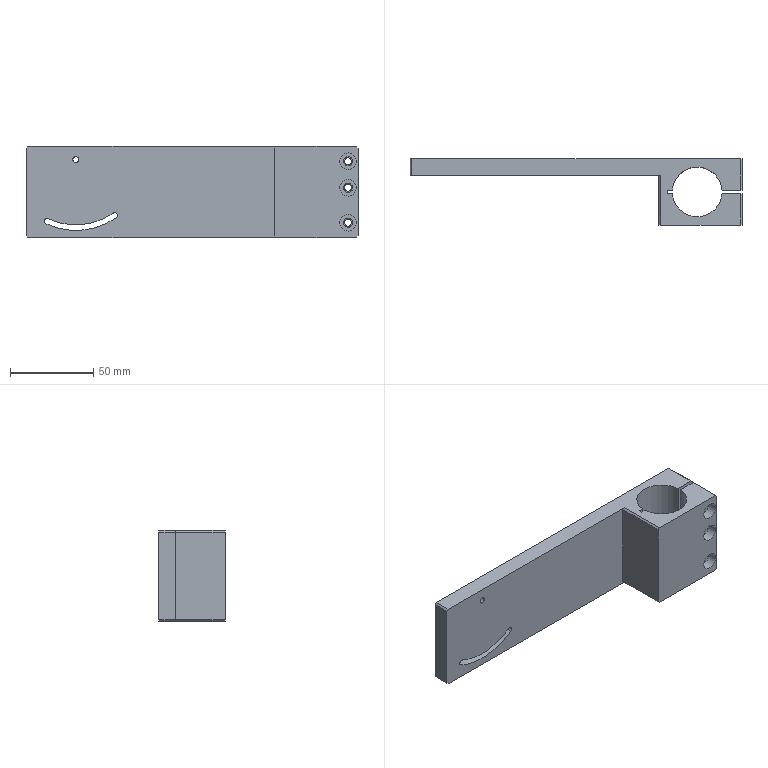Part | 1 solid | 41 faces | box 200 x 40 x 55 mm | volume 147214 mm3 | plane 25 | cylinder 16 | commonest cylinder face diameters 4.2 x3 5.5 x3 10 x3 3.3 x2 30 x2 3.5 x1
STEP:
#1=CARTESIAN_POINT('',(51.,10.,0.));
#2=VERTEX_POINT('',#1);
#3=CARTESIAN_POINT('',(50.,10.,1.));
#4=VERTEX_POINT('',#3);
#5=CARTESIAN_POINT('',(53.5,10.,-2.5));
#6=DIRECTION('',(-0.7071,0.,0.7071));
#7=VECTOR('',#6,1000.);
#8=LINE('',#5,#7);
#9=EDGE_CURVE('',#2,#4,#8,.T.);
#10=ORIENTED_EDGE('',*,*,#9,.F.);
#11=CARTESIAN_POINT('',(51.,-20.,0.));
#12=VERTEX_POINT('',#11);
#13=CARTESIAN_POINT('',(51.,10.,0.));
#14=DIRECTION('',(0.,1.,0.));
#15=VECTOR('',#14,1000.);
#16=LINE('',#13,#15);
#17=EDGE_CURVE('',#12,#2,#16,.T.);
#18=ORIENTED_EDGE('',*,*,#17,.F.);
#19=CARTESIAN_POINT('',(50.,-20.,1.));
#20=VERTEX_POINT('',#19);
#21=CARTESIAN_POINT('',(50.,-20.,1.));
#22=DIRECTION('',(0.7071,0.,-0.7071));
#23=VECTOR('',#22,1000.);
#24=LINE('',#21,#23);
#25=EDGE_CURVE('',#20,#12,#24,.T.);
#26=ORIENTED_EDGE('',*,*,#25,.F.);
#27=CARTESIAN_POINT('',(50.,-20.,1.));
#28=DIRECTION('',(0.,-1.,0.));
#29=VECTOR('',#28,1000.);
#30=LINE('',#27,#29);
#31=EDGE_CURVE('',#4,#20,#30,.T.);
#32=ORIENTED_EDGE('',*,*,#31,.F.);
#33=EDGE_LOOP('',(#10,#18,#26,#32));
#34=FACE_BOUND('',#33,.T.);
#35=CARTESIAN_POINT('',(50.,-20.,1.));
#36=DIRECTION('',(-0.7071,0.,-0.7071));
#37=DIRECTION('',(0.,1.,0.));
#38=AXIS2_PLACEMENT_3D('',#35,#36,#37);
#39=PLANE('',#38);
#40=ADVANCED_FACE('',(#34),#39,.T.);
#41=CARTESIAN_POINT('',(51.,-20.,55.));
#42=VERTEX_POINT('',#41);
#43=CARTESIAN_POINT('',(50.,-20.,54.));
#44=VERTEX_POINT('',#43);
#45=CARTESIAN_POINT('',(50.,-20.,54.));
#46=DIRECTION('',(-0.7071,0.,-0.7071));
#47=VECTOR('',#46,1000.);
#48=LINE('',#45,#47);
#49=EDGE_CURVE('',#42,#44,#48,.T.);
#50=ORIENTED_EDGE('',*,*,#49,.F.);
#51=CARTESIAN_POINT('',(51.,10.,55.));
#52=VERTEX_POINT('',#51);
#53=CARTESIAN_POINT('',(51.,0.,55.));
#54=DIRECTION('',(0.,-1.,0.));
#55=VECTOR('',#54,1000.);
#56=LINE('',#53,#55);
#57=EDGE_CURVE('',#52,#42,#56,.T.);
#58=ORIENTED_EDGE('',*,*,#57,.F.);
#59=CARTESIAN_POINT('',(50.,10.,54.));
#60=VERTEX_POINT('',#59);
#61=CARTESIAN_POINT('',(20.,10.,24.));
#62=DIRECTION('',(0.7071,0.,0.7071));
#63=VECTOR('',#62,1000.);
#64=LINE('',#61,#63);
#65=EDGE_CURVE('',#60,#52,#64,.T.);
#66=ORIENTED_EDGE('',*,*,#65,.F.);
#67=CARTESIAN_POINT('',(50.,-20.,54.));
#68=DIRECTION('',(0.,1.,0.));
#69=VECTOR('',#68,1000.);
#70=LINE('',#67,#69);
#71=EDGE_CURVE('',#44,#60,#70,.T.);
#72=ORIENTED_EDGE('',*,*,#71,.F.);
#73=EDGE_LOOP('',(#50,#58,#66,#72));
#74=FACE_BOUND('',#73,.T.);
#75=CARTESIAN_POINT('',(50.,-20.,54.));
#76=DIRECTION('',(0.7071,0.,-0.7071));
#77=DIRECTION('',(0.,1.,0.));
#78=AXIS2_PLACEMENT_3D('',#75,#76,#77);
#79=PLANE('',#78);
#80=ADVANCED_FACE('',(#74),#79,.F.);
#81=CARTESIAN_POINT('',(-47.441,20.,14.783));
#82=VERTEX_POINT('',#81);
#83=CARTESIAN_POINT('',(-47.441,10.,14.783));
#84=VERTEX_POINT('',#83);
#85=CARTESIAN_POINT('',(-47.441,71.,14.783));
#86=DIRECTION('',(0.,-1.,0.));
#87=VECTOR('',#86,1000.);
#88=LINE('',#85,#87);
#89=EDGE_CURVE('',#82,#84,#88,.T.);
#90=ORIENTED_EDGE('',*,*,#89,.T.);
#91=CARTESIAN_POINT('',(-86.622,10.,11.355));
#92=VERTEX_POINT('',#91);
#93=CARTESIAN_POINT('',(-70.,10.,47.));
#94=DIRECTION('',(0.,1.,0.));
#95=DIRECTION('',(1.,0.,0.));
#96=AXIS2_PLACEMENT_3D('',#93,#94,#95);
#97=CIRCLE('',#96,39.33);
#98=EDGE_CURVE('',#84,#92,#97,.T.);
#99=ORIENTED_EDGE('',*,*,#98,.T.);
#100=CARTESIAN_POINT('',(-86.622,20.,11.355));
#101=VERTEX_POINT('',#100);
#102=CARTESIAN_POINT('',(-86.622,71.,11.355));
#103=DIRECTION('',(0.,-1.,0.));
#104=VECTOR('',#103,1000.);
#105=LINE('',#102,#104);
#106=EDGE_CURVE('',#101,#92,#105,.T.);
#107=ORIENTED_EDGE('',*,*,#106,.F.);
#108=CARTESIAN_POINT('',(-70.,20.,47.));
#109=DIRECTION('',(0.,1.,0.));
#110=DIRECTION('',(0.,0.,-1.));
#111=AXIS2_PLACEMENT_3D('',#108,#109,#110);
#112=CIRCLE('',#111,39.33);
#113=EDGE_CURVE('',#82,#101,#112,.T.);
#114=ORIENTED_EDGE('',*,*,#113,.F.);
#115=EDGE_LOOP('',(#90,#99,#107,#114));
#116=FACE_BOUND('',#115,.T.);
#117=CARTESIAN_POINT('',(-70.,71.,47.));
#118=DIRECTION('',(0.,-1.,0.));
#119=DIRECTION('',(1.,0.,0.));
#120=AXIS2_PLACEMENT_3D('',#117,#118,#119);
#121=CYLINDRICAL_SURFACE('',#120,39.33);
#122=ADVANCED_FACE('',(#116),#121,.T.);
#123=ORIENTED_EDGE('',*,*,#106,.T.);
#124=CARTESIAN_POINT('',(-88.016,10.,8.364));
#125=VERTEX_POINT('',#124);
#126=CARTESIAN_POINT('',(-87.319,10.,9.86));
#127=DIRECTION('',(0.,-1.,0.));
#128=DIRECTION('',(1.,0.,0.));
#129=AXIS2_PLACEMENT_3D('',#126,#127,#128);
#130=CIRCLE('',#129,1.65);
#131=EDGE_CURVE('',#92,#125,#130,.T.);
#132=ORIENTED_EDGE('',*,*,#131,.T.);
#133=CARTESIAN_POINT('',(-88.016,20.,8.364));
#134=VERTEX_POINT('',#133);
#135=CARTESIAN_POINT('',(-88.016,71.,8.364));
#136=DIRECTION('',(0.,-1.,0.));
#137=VECTOR('',#136,1000.);
#138=LINE('',#135,#137);
#139=EDGE_CURVE('',#134,#125,#138,.T.);
#140=ORIENTED_EDGE('',*,*,#139,.F.);
#141=CARTESIAN_POINT('',(-87.319,20.,9.86));
#142=DIRECTION('',(0.,-1.,0.));
#143=DIRECTION('',(0.,0.,-1.));
#144=AXIS2_PLACEMENT_3D('',#141,#142,#143);
#145=CIRCLE('',#144,1.65);
#146=EDGE_CURVE('',#101,#134,#145,.T.);
#147=ORIENTED_EDGE('',*,*,#146,.F.);
#148=EDGE_LOOP('',(#123,#132,#140,#147));
#149=FACE_BOUND('',#148,.T.);
#150=CARTESIAN_POINT('',(-87.319,71.,9.86));
#151=DIRECTION('',(0.,-1.,0.));
#152=DIRECTION('',(1.,0.,0.));
#153=AXIS2_PLACEMENT_3D('',#150,#151,#152);
#154=CYLINDRICAL_SURFACE('',#153,1.65);
#155=ADVANCED_FACE('',(#149),#154,.F.);
#156=ORIENTED_EDGE('',*,*,#139,.T.);
#157=CARTESIAN_POINT('',(-45.548,10.,12.08));
#158=VERTEX_POINT('',#157);
#159=CARTESIAN_POINT('',(-70.,10.,47.));
#160=DIRECTION('',(0.,-1.,0.));
#161=DIRECTION('',(1.,0.,0.));
#162=AXIS2_PLACEMENT_3D('',#159,#160,#161);
#163=CIRCLE('',#162,42.63);
#164=EDGE_CURVE('',#125,#158,#163,.T.);
#165=ORIENTED_EDGE('',*,*,#164,.T.);
#166=CARTESIAN_POINT('',(-45.548,20.,12.08));
#167=VERTEX_POINT('',#166);
#168=CARTESIAN_POINT('',(-45.548,71.,12.08));
#169=DIRECTION('',(0.,-1.,0.));
#170=VECTOR('',#169,1000.);
#171=LINE('',#168,#170);
#172=EDGE_CURVE('',#167,#158,#171,.T.);
#173=ORIENTED_EDGE('',*,*,#172,.F.);
#174=CARTESIAN_POINT('',(-70.,20.,47.));
#175=DIRECTION('',(0.,-1.,0.));
#176=DIRECTION('',(0.,0.,-1.));
#177=AXIS2_PLACEMENT_3D('',#174,#175,#176);
#178=CIRCLE('',#177,42.63);
#179=EDGE_CURVE('',#134,#167,#178,.T.);
#180=ORIENTED_EDGE('',*,*,#179,.F.);
#181=EDGE_LOOP('',(#156,#165,#173,#180));
#182=FACE_BOUND('',#181,.T.);
#183=CARTESIAN_POINT('',(-70.,71.,47.));
#184=DIRECTION('',(0.,-1.,0.));
#185=DIRECTION('',(1.,0.,0.));
#186=AXIS2_PLACEMENT_3D('',#183,#184,#185);
#187=CYLINDRICAL_SURFACE('',#186,42.63);
#188=ADVANCED_FACE('',(#182),#187,.F.);
#189=CARTESIAN_POINT('',(50.,-20.,-6.));
#190=DIRECTION('',(0.,0.,1.));
#191=VECTOR('',#190,1000.);
#192=LINE('',#189,#191);
#193=EDGE_CURVE('',#20,#44,#192,.T.);
#194=ORIENTED_EDGE('',*,*,#193,.T.);
#195=ORIENTED_EDGE('',*,*,#71,.T.);
#196=CARTESIAN_POINT('',(50.,10.,-6.));
#197=DIRECTION('',(0.,0.,1.));
#198=VECTOR('',#197,1000.);
#199=LINE('',#196,#198);
#200=EDGE_CURVE('',#4,#60,#199,.T.);
#201=ORIENTED_EDGE('',*,*,#200,.F.);
#202=ORIENTED_EDGE('',*,*,#31,.T.);
#203=EDGE_LOOP('',(#194,#195,#201,#202));
#204=FACE_BOUND('',#203,.T.);
#205=CARTESIAN_POINT('',(50.,-20.,-6.));
#206=DIRECTION('',(1.,0.,0.));
#207=DIRECTION('',(0.,1.,0.));
#208=AXIS2_PLACEMENT_3D('',#205,#206,#207);
#209=PLANE('',#208);
#210=ADVANCED_FACE('',(#204),#209,.F.);
#211=CARTESIAN_POINT('',(100.,1.,54.));
#212=VERTEX_POINT('',#211);
#213=CARTESIAN_POINT('',(99.,1.,55.));
#214=VERTEX_POINT('',#213);
#215=CARTESIAN_POINT('',(99.,1.,55.));
#216=DIRECTION('',(-0.7071,0.,0.7071));
#217=VECTOR('',#216,1000.);
#218=LINE('',#215,#217);
#219=EDGE_CURVE('',#212,#214,#218,.T.);
#220=ORIENTED_EDGE('',*,*,#219,.F.);
#221=CARTESIAN_POINT('',(100.,20.,54.));
#222=VERTEX_POINT('',#221);
#223=CARTESIAN_POINT('',(100.,-20.,54.));
#224=DIRECTION('',(0.,-1.,0.));
#225=VECTOR('',#224,1000.);
#226=LINE('',#223,#225);
#227=EDGE_CURVE('',#222,#212,#226,.T.);
#228=ORIENTED_EDGE('',*,*,#227,.F.);
#229=CARTESIAN_POINT('',(99.,20.,55.));
#230=VERTEX_POINT('',#229);
#231=CARTESIAN_POINT('',(99.,20.,55.));
#232=DIRECTION('',(0.7071,0.,-0.7071));
#233=VECTOR('',#232,1000.);
#234=LINE('',#231,#233);
#235=EDGE_CURVE('',#230,#222,#234,.T.);
#236=ORIENTED_EDGE('',*,*,#235,.F.);
#237=CARTESIAN_POINT('',(99.,0.,55.));
#238=DIRECTION('',(0.,1.,0.));
#239=VECTOR('',#238,1000.);
#240=LINE('',#237,#239);
#241=EDGE_CURVE('',#214,#230,#240,.T.);
#242=ORIENTED_EDGE('',*,*,#241,.F.);
#243=EDGE_LOOP('',(#220,#228,#236,#242));
#244=FACE_BOUND('',#243,.T.);
#245=CARTESIAN_POINT('',(99.,0.,55.));
#246=DIRECTION('',(-0.7071,0.,-0.7071));
#247=DIRECTION('',(0.,1.,0.));
#248=AXIS2_PLACEMENT_3D('',#245,#246,#247);
#249=PLANE('',#248);
#250=ADVANCED_FACE('',(#244),#249,.F.);
#251=CARTESIAN_POINT('',(100.,-20.,54.));
#252=VERTEX_POINT('',#251);
#253=CARTESIAN_POINT('',(99.,-20.,55.));
#254=VERTEX_POINT('',#253);
#255=CARTESIAN_POINT('',(99.,-20.,55.));
#256=DIRECTION('',(-0.7071,0.,0.7071));
#257=VECTOR('',#256,1000.);
#258=LINE('',#255,#257);
#259=EDGE_CURVE('',#252,#254,#258,.T.);
#260=ORIENTED_EDGE('',*,*,#259,.F.);
#261=CARTESIAN_POINT('',(100.,-1.,54.));
#262=VERTEX_POINT('',#261);
#263=CARTESIAN_POINT('',(100.,-20.,54.));
#264=DIRECTION('',(0.,-1.,0.));
#265=VECTOR('',#264,1000.);
#266=LINE('',#263,#265);
#267=EDGE_CURVE('',#262,#252,#266,.T.);
#268=ORIENTED_EDGE('',*,*,#267,.F.);
#269=CARTESIAN_POINT('',(99.,-1.,55.));
#270=VERTEX_POINT('',#269);
#271=CARTESIAN_POINT('',(99.,-1.,55.));
#272=DIRECTION('',(0.7071,0.,-0.7071));
#273=VECTOR('',#272,1000.);
#274=LINE('',#271,#273);
#275=EDGE_CURVE('',#270,#262,#274,.T.);
#276=ORIENTED_EDGE('',*,*,#275,.F.);
#277=CARTESIAN_POINT('',(99.,0.,55.));
#278=DIRECTION('',(0.,1.,0.));
#279=VECTOR('',#278,1000.);
#280=LINE('',#277,#279);
#281=EDGE_CURVE('',#254,#270,#280,.T.);
#282=ORIENTED_EDGE('',*,*,#281,.F.);
#283=EDGE_LOOP('',(#260,#268,#276,#282));
#284=FACE_BOUND('',#283,.T.);
#285=CARTESIAN_POINT('',(99.,0.,55.));
#286=DIRECTION('',(-0.7071,0.,-0.7071));
#287=DIRECTION('',(0.,1.,0.));
#288=AXIS2_PLACEMENT_3D('',#285,#286,#287);
#289=PLANE('',#288);
#290=ADVANCED_FACE('',(#284),#289,.F.);
#291=CARTESIAN_POINT('',(99.,1.,0.));
#292=VERTEX_POINT('',#291);
#293=CARTESIAN_POINT('',(100.,1.,1.));
#294=VERTEX_POINT('',#293);
#295=CARTESIAN_POINT('',(100.,1.,1.));
#296=DIRECTION('',(0.7071,0.,0.7071));
#297=VECTOR('',#296,1000.);
#298=LINE('',#295,#297);
#299=EDGE_CURVE('',#292,#294,#298,.T.);
#300=ORIENTED_EDGE('',*,*,#299,.F.);
#301=CARTESIAN_POINT('',(99.,20.,0.));
#302=VERTEX_POINT('',#301);
#303=CARTESIAN_POINT('',(99.,1.,0.));
#304=DIRECTION('',(0.,-1.,0.));
#305=VECTOR('',#304,1000.);
#306=LINE('',#303,#305);
#307=EDGE_CURVE('',#302,#292,#306,.T.);
#308=ORIENTED_EDGE('',*,*,#307,.F.);
#309=CARTESIAN_POINT('',(100.,20.,1.));
#310=VERTEX_POINT('',#309);
#311=CARTESIAN_POINT('',(100.,20.,1.));
#312=DIRECTION('',(-0.7071,0.,-0.7071));
#313=VECTOR('',#312,1000.);
#314=LINE('',#311,#313);
#315=EDGE_CURVE('',#310,#302,#314,.T.);
#316=ORIENTED_EDGE('',*,*,#315,.F.);
#317=CARTESIAN_POINT('',(100.,20.,1.));
#318=DIRECTION('',(0.,1.,0.));
#319=VECTOR('',#318,1000.);
#320=LINE('',#317,#319);
#321=EDGE_CURVE('',#294,#310,#320,.T.);
#322=ORIENTED_EDGE('',*,*,#321,.F.);
#323=EDGE_LOOP('',(#300,#308,#316,#322));
#324=FACE_BOUND('',#323,.T.);
#325=CARTESIAN_POINT('',(100.,-20.,1.));
#326=DIRECTION('',(0.7071,0.,-0.7071));
#327=DIRECTION('',(0.,-1.,0.));
#328=AXIS2_PLACEMENT_3D('',#325,#326,#327);
#329=PLANE('',#328);
#330=ADVANCED_FACE('',(#324),#329,.T.);
#331=CARTESIAN_POINT('',(99.,-20.,0.));
#332=VERTEX_POINT('',#331);
#333=CARTESIAN_POINT('',(100.,-20.,1.));
#334=VERTEX_POINT('',#333);
#335=CARTESIAN_POINT('',(100.,-20.,1.));
#336=DIRECTION('',(0.7071,0.,0.7071));
#337=VECTOR('',#336,1000.);
#338=LINE('',#335,#337);
#339=EDGE_CURVE('',#332,#334,#338,.T.);
#340=ORIENTED_EDGE('',*,*,#339,.F.);
#341=CARTESIAN_POINT('',(99.,-1.,0.));
#342=VERTEX_POINT('',#341);
#343=CARTESIAN_POINT('',(99.,-20.,0.));
#344=DIRECTION('',(0.,-1.,0.));
#345=VECTOR('',#344,1000.);
#346=LINE('',#343,#345);
#347=EDGE_CURVE('',#342,#332,#346,.T.);
#348=ORIENTED_EDGE('',*,*,#347,.F.);
#349=CARTESIAN_POINT('',(100.,-1.,1.));
#350=VERTEX_POINT('',#349);
#351=CARTESIAN_POINT('',(100.,-1.,1.));
#352=DIRECTION('',(-0.7071,0.,-0.7071));
#353=VECTOR('',#352,1000.);
#354=LINE('',#351,#353);
#355=EDGE_CURVE('',#350,#342,#354,.T.);
#356=ORIENTED_EDGE('',*,*,#355,.F.);
#357=CARTESIAN_POINT('',(100.,-1.,1.));
#358=DIRECTION('',(0.,1.,0.));
#359=VECTOR('',#358,1000.);
#360=LINE('',#357,#359);
#361=EDGE_CURVE('',#334,#350,#360,.T.);
#362=ORIENTED_EDGE('',*,*,#361,.F.);
#363=EDGE_LOOP('',(#340,#348,#356,#362));
#364=FACE_BOUND('',#363,.T.);
#365=CARTESIAN_POINT('',(100.,-20.,1.));
#366=DIRECTION('',(0.7071,0.,-0.7071));
#367=DIRECTION('',(0.,-1.,0.));
#368=AXIS2_PLACEMENT_3D('',#365,#366,#367);
#369=PLANE('',#368);
#370=ADVANCED_FACE('',(#364),#369,.T.);
#371=CARTESIAN_POINT('',(-99.,10.,55.));
#372=VERTEX_POINT('',#371);
#373=CARTESIAN_POINT('',(-100.,10.,54.));
#374=VERTEX_POINT('',#373);
#375=CARTESIAN_POINT('',(-99.,10.,55.));
#376=DIRECTION('',(-0.7071,0.,-0.7071));
#377=VECTOR('',#376,1000.);
#378=LINE('',#375,#377);
#379=EDGE_CURVE('',#372,#374,#378,.T.);
#380=ORIENTED_EDGE('',*,*,#379,.F.);
#381=CARTESIAN_POINT('',(-99.,20.,55.));
#382=VERTEX_POINT('',#381);
#383=CARTESIAN_POINT('',(-99.,0.,55.));
#384=DIRECTION('',(0.,-1.,0.));
#385=VECTOR('',#384,1000.);
#386=LINE('',#383,#385);
#387=EDGE_CURVE('',#382,#372,#386,.T.);
#388=ORIENTED_EDGE('',*,*,#387,.F.);
#389=CARTESIAN_POINT('',(-100.,20.,54.));
#390=VERTEX_POINT('',#389);
#391=CARTESIAN_POINT('',(-99.,20.,55.));
#392=DIRECTION('',(0.7071,0.,0.7071));
#393=VECTOR('',#392,1000.);
#394=LINE('',#391,#393);
#395=EDGE_CURVE('',#390,#382,#394,.T.);
#396=ORIENTED_EDGE('',*,*,#395,.F.);
#397=CARTESIAN_POINT('',(-100.,-20.,54.));
#398=DIRECTION('',(0.,1.,0.));
#399=VECTOR('',#398,1000.);
#400=LINE('',#397,#399);
#401=EDGE_CURVE('',#374,#390,#400,.T.);
#402=ORIENTED_EDGE('',*,*,#401,.F.);
#403=EDGE_LOOP('',(#380,#388,#396,#402));
#404=FACE_BOUND('',#403,.T.);
#405=CARTESIAN_POINT('',(-99.,0.,55.));
#406=DIRECTION('',(0.7071,0.,-0.7071));
#407=DIRECTION('',(0.,-1.,0.));
#408=AXIS2_PLACEMENT_3D('',#405,#406,#407);
#409=PLANE('',#408);
#410=ADVANCED_FACE('',(#404),#409,.F.);
#411=CARTESIAN_POINT('',(-100.,10.,1.));
#412=VERTEX_POINT('',#411);
#413=CARTESIAN_POINT('',(-99.,10.,0.));
#414=VERTEX_POINT('',#413);
#415=CARTESIAN_POINT('',(-100.,10.,1.));
#416=DIRECTION('',(0.7071,0.,-0.7071));
#417=VECTOR('',#416,1000.);
#418=LINE('',#415,#417);
#419=EDGE_CURVE('',#412,#414,#418,.T.);
#420=ORIENTED_EDGE('',*,*,#419,.F.);
#421=CARTESIAN_POINT('',(-100.,20.,1.));
#422=VERTEX_POINT('',#421);
#423=CARTESIAN_POINT('',(-100.,-20.,1.));
#424=DIRECTION('',(0.,-1.,0.));
#425=VECTOR('',#424,1000.);
#426=LINE('',#423,#425);
#427=EDGE_CURVE('',#422,#412,#426,.T.);
#428=ORIENTED_EDGE('',*,*,#427,.F.);
#429=CARTESIAN_POINT('',(-99.,20.,0.));
#430=VERTEX_POINT('',#429);
#431=CARTESIAN_POINT('',(-100.,20.,1.));
#432=DIRECTION('',(-0.7071,0.,0.7071));
#433=VECTOR('',#432,1000.);
#434=LINE('',#431,#433);
#435=EDGE_CURVE('',#430,#422,#434,.T.);
#436=ORIENTED_EDGE('',*,*,#435,.F.);
#437=CARTESIAN_POINT('',(-99.,20.,0.));
#438=DIRECTION('',(0.,1.,0.));
#439=VECTOR('',#438,1000.);
#440=LINE('',#437,#439);
#441=EDGE_CURVE('',#414,#430,#440,.T.);
#442=ORIENTED_EDGE('',*,*,#441,.F.);
#443=EDGE_LOOP('',(#420,#428,#436,#442));
#444=FACE_BOUND('',#443,.T.);
#445=CARTESIAN_POINT('',(-100.,-20.,1.));
#446=DIRECTION('',(-0.7071,0.,-0.7071));
#447=DIRECTION('',(0.,1.,0.));
#448=AXIS2_PLACEMENT_3D('',#445,#446,#447);
#449=PLANE('',#448);
#450=ADVANCED_FACE('',(#444),#449,.T.);
#451=CARTESIAN_POINT('',(94.,-14.3,41.));
#452=VERTEX_POINT('',#451);
#453=CARTESIAN_POINT('',(94.,-14.3,46.));
#454=DIRECTION('',(0.,-1.,0.));
#455=DIRECTION('',(0.,0.,-1.));
#456=AXIS2_PLACEMENT_3D('',#453,#454,#455);
#457=CIRCLE('',#456,5.);
#458=EDGE_CURVE('',#452,#452,#457,.T.);
#459=ORIENTED_EDGE('',*,*,#458,.T.);
#460=EDGE_LOOP('',(#459));
#461=FACE_BOUND('',#460,.T.);
#462=CARTESIAN_POINT('',(94.,-14.3,43.25));
#463=VERTEX_POINT('',#462);
#464=CARTESIAN_POINT('',(94.,-14.3,46.));
#465=DIRECTION('',(0.,-1.,0.));
#466=DIRECTION('',(0.,0.,-1.));
#467=AXIS2_PLACEMENT_3D('',#464,#465,#466);
#468=CIRCLE('',#467,2.75);
#469=EDGE_CURVE('',#463,#463,#468,.T.);
#470=ORIENTED_EDGE('',*,*,#469,.F.);
#471=EDGE_LOOP('',(#470));
#472=FACE_BOUND('',#471,.T.);
#473=CARTESIAN_POINT('',(96.75,-14.3,46.));
#474=DIRECTION('',(0.,1.,0.));
#475=DIRECTION('',(0.,0.,1.));
#476=AXIS2_PLACEMENT_3D('',#473,#474,#475);
#477=PLANE('',#476);
#478=ADVANCED_FACE('',(#461,#472),#477,.F.);
#479=CARTESIAN_POINT('',(94.,-14.3,14.));
#480=VERTEX_POINT('',#479);
#481=CARTESIAN_POINT('',(94.,-14.3,9.));
#482=DIRECTION('',(0.,-1.,0.));
#483=DIRECTION('',(0.,0.,1.));
#484=AXIS2_PLACEMENT_3D('',#481,#482,#483);
#485=CIRCLE('',#484,5.);
#486=EDGE_CURVE('',#480,#480,#485,.T.);
#487=ORIENTED_EDGE('',*,*,#486,.T.);
#488=EDGE_LOOP('',(#487));
#489=FACE_BOUND('',#488,.T.);
#490=CARTESIAN_POINT('',(94.,-14.3,11.75));
#491=VERTEX_POINT('',#490);
#492=CARTESIAN_POINT('',(94.,-14.3,9.));
#493=DIRECTION('',(0.,-1.,0.));
#494=DIRECTION('',(0.,0.,1.));
#495=AXIS2_PLACEMENT_3D('',#492,#493,#494);
#496=CIRCLE('',#495,2.75);
#497=EDGE_CURVE('',#491,#491,#496,.T.);
#498=ORIENTED_EDGE('',*,*,#497,.F.);
#499=EDGE_LOOP('',(#498));
#500=FACE_BOUND('',#499,.T.);
#501=CARTESIAN_POINT('',(96.75,-14.3,46.));
#502=DIRECTION('',(0.,1.,0.));
#503=DIRECTION('',(0.,0.,1.));
#504=AXIS2_PLACEMENT_3D('',#501,#502,#503);
#505=PLANE('',#504);
#506=ADVANCED_FACE('',(#489,#500),#505,.F.);
#507=CARTESIAN_POINT('',(94.,-14.3,35.));
#508=VERTEX_POINT('',#507);
#509=CARTESIAN_POINT('',(94.,-14.3,30.));
#510=DIRECTION('',(0.,-1.,0.));
#511=DIRECTION('',(0.,0.,1.));
#512=AXIS2_PLACEMENT_3D('',#509,#510,#511);
#513=CIRCLE('',#512,5.);
#514=EDGE_CURVE('',#508,#508,#513,.T.);
#515=ORIENTED_EDGE('',*,*,#514,.T.);
#516=EDGE_LOOP('',(#515));
#517=FACE_BOUND('',#516,.T.);
#518=CARTESIAN_POINT('',(94.,-14.3,32.75));
#519=VERTEX_POINT('',#518);
#520=CARTESIAN_POINT('',(94.,-14.3,30.));
#521=DIRECTION('',(0.,-1.,0.));
#522=DIRECTION('',(0.,0.,1.));
#523=AXIS2_PLACEMENT_3D('',#520,#521,#522);
#524=CIRCLE('',#523,2.75);
#525=EDGE_CURVE('',#519,#519,#524,.T.);
#526=ORIENTED_EDGE('',*,*,#525,.F.);
#527=EDGE_LOOP('',(#526));
#528=FACE_BOUND('',#527,.T.);
#529=CARTESIAN_POINT('',(96.75,-14.3,46.));
#530=DIRECTION('',(0.,1.,0.));
#531=DIRECTION('',(0.,0.,1.));
#532=AXIS2_PLACEMENT_3D('',#529,#530,#531);
#533=PLANE('',#532);
#534=ADVANCED_FACE('',(#517,#528),#533,.F.);
#535=CARTESIAN_POINT('',(55.,-1.,0.));
#536=VERTEX_POINT('',#535);
#537=CARTESIAN_POINT('',(55.,1.,0.));
#538=VERTEX_POINT('',#537);
#539=CARTESIAN_POINT('',(55.,0.,0.));
#540=DIRECTION('',(0.,1.,0.));
#541=VECTOR('',#540,1000.);
#542=LINE('',#539,#541);
#543=EDGE_CURVE('',#536,#538,#542,.T.);
#544=ORIENTED_EDGE('',*,*,#543,.T.);
#545=CARTESIAN_POINT('',(55.,1.,55.));
#546=VERTEX_POINT('',#545);
#547=CARTESIAN_POINT('',(55.,1.,-5.));
#548=DIRECTION('',(0.,0.,1.));
#549=VECTOR('',#548,1000.);
#550=LINE('',#547,#549);
#551=EDGE_CURVE('',#538,#546,#550,.T.);
#552=ORIENTED_EDGE('',*,*,#551,.T.);
#553=CARTESIAN_POINT('',(55.,-1.,55.));
#554=VERTEX_POINT('',#553);
#555=CARTESIAN_POINT('',(55.,1.,55.));
#556=DIRECTION('',(0.,-1.,0.));
#557=VECTOR('',#556,1000.);
#558=LINE('',#555,#557);
#559=EDGE_CURVE('',#546,#554,#558,.T.);
#560=ORIENTED_EDGE('',*,*,#559,.T.);
#561=CARTESIAN_POINT('',(55.,-1.,-5.));
#562=DIRECTION('',(0.,0.,1.));
#563=VECTOR('',#562,1000.);
#564=LINE('',#561,#563);
#565=EDGE_CURVE('',#536,#554,#564,.T.);
#566=ORIENTED_EDGE('',*,*,#565,.F.);
#567=EDGE_LOOP('',(#544,#552,#560,#566));
#568=FACE_BOUND('',#567,.T.);
#569=CARTESIAN_POINT('',(55.,1.,-5.));
#570=DIRECTION('',(-1.,0.,0.));
#571=DIRECTION('',(0.,0.,1.));
#572=AXIS2_PLACEMENT_3D('',#569,#570,#571);
#573=PLANE('',#572);
#574=ADVANCED_FACE('',(#568),#573,.F.);
#575=CARTESIAN_POINT('',(58.033,-1.,0.));
#576=VERTEX_POINT('',#575);
#577=CARTESIAN_POINT('',(0.,-1.,0.));
#578=DIRECTION('',(-1.,0.,0.));
#579=VECTOR('',#578,1000.);
#580=LINE('',#577,#579);
#581=EDGE_CURVE('',#576,#536,#580,.T.);
#582=ORIENTED_EDGE('',*,*,#581,.T.);
#583=ORIENTED_EDGE('',*,*,#565,.T.);
#584=CARTESIAN_POINT('',(58.033,-1.,55.));
#585=VERTEX_POINT('',#584);
#586=CARTESIAN_POINT('',(100.,-1.,55.));
#587=DIRECTION('',(1.,0.,0.));
#588=VECTOR('',#587,1000.);
#589=LINE('',#586,#588);
#590=EDGE_CURVE('',#554,#585,#589,.T.);
#591=ORIENTED_EDGE('',*,*,#590,.T.);
#592=CARTESIAN_POINT('',(58.033,-1.,-7.));
#593=DIRECTION('',(0.,0.,1.));
#594=VECTOR('',#593,1000.);
#595=LINE('',#592,#594);
#596=EDGE_CURVE('',#576,#585,#595,.T.);
#597=ORIENTED_EDGE('',*,*,#596,.F.);
#598=EDGE_LOOP('',(#582,#583,#591,#597));
#599=FACE_BOUND('',#598,.T.);
#600=CARTESIAN_POINT('',(100.,-1.,-5.));
#601=DIRECTION('',(0.,-1.,0.));
#602=DIRECTION('',(1.,0.,0.));
#603=AXIS2_PLACEMENT_3D('',#600,#601,#602);
#604=PLANE('',#603);
#605=ADVANCED_FACE('',(#599),#604,.F.);
#606=CARTESIAN_POINT('',(58.033,1.,0.));
#607=VERTEX_POINT('',#606);
#608=CARTESIAN_POINT('',(0.,1.,0.));
#609=DIRECTION('',(1.,0.,0.));
#610=VECTOR('',#609,1000.);
#611=LINE('',#608,#610);
#612=EDGE_CURVE('',#538,#607,#611,.T.);
#613=ORIENTED_EDGE('',*,*,#612,.T.);
#614=CARTESIAN_POINT('',(58.033,1.,55.));
#615=VERTEX_POINT('',#614);
#616=CARTESIAN_POINT('',(58.033,1.,-7.));
#617=DIRECTION('',(0.,0.,-1.));
#618=VECTOR('',#617,1000.);
#619=LINE('',#616,#618);
#620=EDGE_CURVE('',#615,#607,#619,.T.);
#621=ORIENTED_EDGE('',*,*,#620,.F.);
#622=CARTESIAN_POINT('',(100.,1.,55.));
#623=DIRECTION('',(-1.,0.,0.));
#624=VECTOR('',#623,1000.);
#625=LINE('',#622,#624);
#626=EDGE_CURVE('',#615,#546,#625,.T.);
#627=ORIENTED_EDGE('',*,*,#626,.T.);
#628=ORIENTED_EDGE('',*,*,#551,.F.);
#629=EDGE_LOOP('',(#613,#621,#627,#628));
#630=FACE_BOUND('',#629,.T.);
#631=CARTESIAN_POINT('',(100.,1.,-5.));
#632=DIRECTION('',(0.,1.,0.));
#633=DIRECTION('',(-1.,0.,0.));
#634=AXIS2_PLACEMENT_3D('',#631,#632,#633);
#635=PLANE('',#634);
#636=ADVANCED_FACE('',(#630),#635,.F.);
#637=CARTESIAN_POINT('',(87.967,1.,0.));
#638=VERTEX_POINT('',#637);
#639=CARTESIAN_POINT('',(0.,1.,0.));
#640=DIRECTION('',(1.,0.,0.));
#641=VECTOR('',#640,1000.);
#642=LINE('',#639,#641);
#643=EDGE_CURVE('',#638,#292,#642,.T.);
#644=ORIENTED_EDGE('',*,*,#643,.T.);
#645=ORIENTED_EDGE('',*,*,#299,.T.);
#646=CARTESIAN_POINT('',(100.,1.,-5.));
#647=DIRECTION('',(0.,0.,1.));
#648=VECTOR('',#647,1000.);
#649=LINE('',#646,#648);
#650=EDGE_CURVE('',#294,#212,#649,.T.);
#651=ORIENTED_EDGE('',*,*,#650,.T.);
#652=ORIENTED_EDGE('',*,*,#219,.T.);
#653=CARTESIAN_POINT('',(87.967,1.,55.));
#654=VERTEX_POINT('',#653);
#655=CARTESIAN_POINT('',(100.,1.,55.));
#656=DIRECTION('',(-1.,0.,0.));
#657=VECTOR('',#656,1000.);
#658=LINE('',#655,#657);
#659=EDGE_CURVE('',#214,#654,#658,.T.);
#660=ORIENTED_EDGE('',*,*,#659,.T.);
#661=CARTESIAN_POINT('',(87.967,1.,-7.));
#662=DIRECTION('',(0.,0.,1.));
#663=VECTOR('',#662,1000.);
#664=LINE('',#661,#663);
#665=EDGE_CURVE('',#638,#654,#664,.T.);
#666=ORIENTED_EDGE('',*,*,#665,.F.);
#667=EDGE_LOOP('',(#644,#645,#651,#652,#660,#666));
#668=FACE_BOUND('',#667,.T.);
#669=CARTESIAN_POINT('',(94.,1.,43.9));
#670=VERTEX_POINT('',#669);
#671=CARTESIAN_POINT('',(94.,1.,46.));
#672=DIRECTION('',(0.,-1.,0.));
#673=DIRECTION('',(0.,0.,-1.));
#674=AXIS2_PLACEMENT_3D('',#671,#672,#673);
#675=CIRCLE('',#674,2.1);
#676=EDGE_CURVE('',#670,#670,#675,.T.);
#677=ORIENTED_EDGE('',*,*,#676,.F.);
#678=EDGE_LOOP('',(#677));
#679=FACE_BOUND('',#678,.T.);
#680=CARTESIAN_POINT('',(94.,1.,27.9));
#681=VERTEX_POINT('',#680);
#682=CARTESIAN_POINT('',(94.,1.,30.));
#683=DIRECTION('',(0.,-1.,0.));
#684=DIRECTION('',(0.,0.,-1.));
#685=AXIS2_PLACEMENT_3D('',#682,#683,#684);
#686=CIRCLE('',#685,2.1);
#687=EDGE_CURVE('',#681,#681,#686,.T.);
#688=ORIENTED_EDGE('',*,*,#687,.F.);
#689=EDGE_LOOP('',(#688));
#690=FACE_BOUND('',#689,.T.);
#691=CARTESIAN_POINT('',(94.,1.,6.9));
#692=VERTEX_POINT('',#691);
#693=CARTESIAN_POINT('',(94.,1.,9.));
#694=DIRECTION('',(0.,-1.,0.));
#695=DIRECTION('',(0.,0.,-1.));
#696=AXIS2_PLACEMENT_3D('',#693,#694,#695);
#697=CIRCLE('',#696,2.1);
#698=EDGE_CURVE('',#692,#692,#697,.T.);
#699=ORIENTED_EDGE('',*,*,#698,.F.);
#700=EDGE_LOOP('',(#699));
#701=FACE_BOUND('',#700,.T.);
#702=CARTESIAN_POINT('',(100.,1.,-5.));
#703=DIRECTION('',(0.,1.,0.));
#704=DIRECTION('',(-1.,0.,0.));
#705=AXIS2_PLACEMENT_3D('',#702,#703,#704);
#706=PLANE('',#705);
#707=ADVANCED_FACE('',(#668,#679,#690,#701),#706,.F.);
#708=CARTESIAN_POINT('',(73.,0.,55.));
#709=DIRECTION('',(0.,0.,1.));
#710=DIRECTION('',(1.,0.,0.));
#711=AXIS2_PLACEMENT_3D('',#708,#709,#710);
#712=CIRCLE('',#711,15.);
#713=EDGE_CURVE('',#654,#615,#712,.T.);
#714=ORIENTED_EDGE('',*,*,#713,.T.);
#715=ORIENTED_EDGE('',*,*,#620,.T.);
#716=CARTESIAN_POINT('',(73.,0.,0.));
#717=DIRECTION('',(0.,0.,-1.));
#718=DIRECTION('',(-1.,0.,0.));
#719=AXIS2_PLACEMENT_3D('',#716,#717,#718);
#720=CIRCLE('',#719,15.);
#721=EDGE_CURVE('',#607,#638,#720,.T.);
#722=ORIENTED_EDGE('',*,*,#721,.T.);
#723=ORIENTED_EDGE('',*,*,#665,.T.);
#724=EDGE_LOOP('',(#714,#715,#722,#723));
#725=FACE_BOUND('',#724,.T.);
#726=CARTESIAN_POINT('',(73.,0.,-7.));
#727=DIRECTION('',(0.,0.,1.));
#728=DIRECTION('',(1.,0.,0.));
#729=AXIS2_PLACEMENT_3D('',#726,#727,#728);
#730=CYLINDRICAL_SURFACE('',#729,15.);
#731=ADVANCED_FACE('',(#725),#730,.F.);
#732=CARTESIAN_POINT('',(-100.,-20.,0.));
#733=DIRECTION('',(1.,0.,0.));
#734=VECTOR('',#733,1000.);
#735=LINE('',#732,#734);
#736=EDGE_CURVE('',#12,#332,#735,.T.);
#737=ORIENTED_EDGE('',*,*,#736,.F.);
#738=ORIENTED_EDGE('',*,*,#17,.T.);
#739=CARTESIAN_POINT('',(0.,10.,0.));
#740=DIRECTION('',(1.,0.,0.));
#741=VECTOR('',#740,1000.);
#742=LINE('',#739,#741);
#743=EDGE_CURVE('',#414,#2,#742,.T.);
#744=ORIENTED_EDGE('',*,*,#743,.F.);
#745=ORIENTED_EDGE('',*,*,#441,.T.);
#746=CARTESIAN_POINT('',(-100.,20.,0.));
#747=DIRECTION('',(-1.,0.,0.));
#748=VECTOR('',#747,1000.);
#749=LINE('',#746,#748);
#750=EDGE_CURVE('',#302,#430,#749,.T.);
#751=ORIENTED_EDGE('',*,*,#750,.F.);
#752=ORIENTED_EDGE('',*,*,#307,.T.);
#753=ORIENTED_EDGE('',*,*,#643,.F.);
#754=ORIENTED_EDGE('',*,*,#721,.F.);
#755=ORIENTED_EDGE('',*,*,#612,.F.);
#756=ORIENTED_EDGE('',*,*,#543,.F.);
#757=ORIENTED_EDGE('',*,*,#581,.F.);
#758=CARTESIAN_POINT('',(87.967,-1.,0.));
#759=VERTEX_POINT('',#758);
#760=CARTESIAN_POINT('',(73.,0.,0.));
#761=DIRECTION('',(0.,0.,-1.));
#762=DIRECTION('',(-1.,0.,0.));
#763=AXIS2_PLACEMENT_3D('',#760,#761,#762);
#764=CIRCLE('',#763,15.);
#765=EDGE_CURVE('',#759,#576,#764,.T.);
#766=ORIENTED_EDGE('',*,*,#765,.F.);
#767=CARTESIAN_POINT('',(0.,-1.,0.));
#768=DIRECTION('',(-1.,0.,0.));
#769=VECTOR('',#768,1000.);
#770=LINE('',#767,#769);
#771=EDGE_CURVE('',#342,#759,#770,.T.);
#772=ORIENTED_EDGE('',*,*,#771,.F.);
#773=ORIENTED_EDGE('',*,*,#347,.T.);
#774=EDGE_LOOP('',(#737,#738,#744,#745,#751,#752,#753,#754,#755,#756,#757,#766,#772,#773));
#775=FACE_BOUND('',#774,.T.);
#776=CARTESIAN_POINT('',(0.,0.,0.));
#777=DIRECTION('',(0.,0.,-1.));
#778=DIRECTION('',(-1.,0.,0.));
#779=AXIS2_PLACEMENT_3D('',#776,#777,#778);
#780=PLANE('',#779);
#781=ADVANCED_FACE('',(#775),#780,.T.);
#782=CARTESIAN_POINT('',(50.,10.,55.));
#783=DIRECTION('',(-1.,0.,0.));
#784=VECTOR('',#783,1000.);
#785=LINE('',#782,#784);
#786=EDGE_CURVE('',#52,#372,#785,.T.);
#787=ORIENTED_EDGE('',*,*,#786,.F.);
#788=ORIENTED_EDGE('',*,*,#57,.T.);
#789=CARTESIAN_POINT('',(-100.,-20.,55.));
#790=DIRECTION('',(1.,0.,0.));
#791=VECTOR('',#790,1000.);
#792=LINE('',#789,#791);
#793=EDGE_CURVE('',#42,#254,#792,.T.);
#794=ORIENTED_EDGE('',*,*,#793,.T.);
#795=ORIENTED_EDGE('',*,*,#281,.T.);
#796=CARTESIAN_POINT('',(87.967,-1.,55.));
#797=VERTEX_POINT('',#796);
#798=CARTESIAN_POINT('',(100.,-1.,55.));
#799=DIRECTION('',(1.,0.,0.));
#800=VECTOR('',#799,1000.);
#801=LINE('',#798,#800);
#802=EDGE_CURVE('',#797,#270,#801,.T.);
#803=ORIENTED_EDGE('',*,*,#802,.F.);
#804=CARTESIAN_POINT('',(73.,0.,55.));
#805=DIRECTION('',(0.,0.,1.));
#806=DIRECTION('',(1.,0.,0.));
#807=AXIS2_PLACEMENT_3D('',#804,#805,#806);
#808=CIRCLE('',#807,15.);
#809=EDGE_CURVE('',#585,#797,#808,.T.);
#810=ORIENTED_EDGE('',*,*,#809,.F.);
#811=ORIENTED_EDGE('',*,*,#590,.F.);
#812=ORIENTED_EDGE('',*,*,#559,.F.);
#813=ORIENTED_EDGE('',*,*,#626,.F.);
#814=ORIENTED_EDGE('',*,*,#713,.F.);
#815=ORIENTED_EDGE('',*,*,#659,.F.);
#816=ORIENTED_EDGE('',*,*,#241,.T.);
#817=CARTESIAN_POINT('',(-100.,20.,55.));
#818=DIRECTION('',(-1.,0.,0.));
#819=VECTOR('',#818,1000.);
#820=LINE('',#817,#819);
#821=EDGE_CURVE('',#230,#382,#820,.T.);
#822=ORIENTED_EDGE('',*,*,#821,.T.);
#823=ORIENTED_EDGE('',*,*,#387,.T.);
#824=EDGE_LOOP('',(#787,#788,#794,#795,#803,#810,#811,#812,#813,#814,#815,#816,#822,#823));
#825=FACE_BOUND('',#824,.T.);
#826=CARTESIAN_POINT('',(0.,0.,55.));
#827=DIRECTION('',(0.,0.,-1.));
#828=DIRECTION('',(-1.,0.,0.));
#829=AXIS2_PLACEMENT_3D('',#826,#827,#828);
#830=PLANE('',#829);
#831=ADVANCED_FACE('',(#825),#830,.F.);
#832=ORIENTED_EDGE('',*,*,#793,.F.);
#833=ORIENTED_EDGE('',*,*,#49,.T.);
#834=ORIENTED_EDGE('',*,*,#193,.F.);
#835=ORIENTED_EDGE('',*,*,#25,.T.);
#836=ORIENTED_EDGE('',*,*,#736,.T.);
#837=ORIENTED_EDGE('',*,*,#339,.T.);
#838=CARTESIAN_POINT('',(100.,-20.,55.));
#839=DIRECTION('',(0.,0.,-1.));
#840=VECTOR('',#839,1000.);
#841=LINE('',#838,#840);
#842=EDGE_CURVE('',#252,#334,#841,.T.);
#843=ORIENTED_EDGE('',*,*,#842,.F.);
#844=ORIENTED_EDGE('',*,*,#259,.T.);
#845=EDGE_LOOP('',(#832,#833,#834,#835,#836,#837,#843,#844));
#846=FACE_BOUND('',#845,.T.);
#847=CARTESIAN_POINT('',(94.,-20.,25.));
#848=VERTEX_POINT('',#847);
#849=CARTESIAN_POINT('',(94.,-20.,30.));
#850=DIRECTION('',(0.,-1.,0.));
#851=DIRECTION('',(0.,0.,-1.));
#852=AXIS2_PLACEMENT_3D('',#849,#850,#851);
#853=CIRCLE('',#852,5.);
#854=EDGE_CURVE('',#848,#848,#853,.T.);
#855=ORIENTED_EDGE('',*,*,#854,.F.);
#856=EDGE_LOOP('',(#855));
#857=FACE_BOUND('',#856,.T.);
#858=CARTESIAN_POINT('',(94.,-20.,4.));
#859=VERTEX_POINT('',#858);
#860=CARTESIAN_POINT('',(94.,-20.,9.));
#861=DIRECTION('',(0.,-1.,0.));
#862=DIRECTION('',(0.,0.,-1.));
#863=AXIS2_PLACEMENT_3D('',#860,#861,#862);
#864=CIRCLE('',#863,5.);
#865=EDGE_CURVE('',#859,#859,#864,.T.);
#866=ORIENTED_EDGE('',*,*,#865,.F.);
#867=EDGE_LOOP('',(#866));
#868=FACE_BOUND('',#867,.T.);
#869=CARTESIAN_POINT('',(94.,-20.,41.));
#870=VERTEX_POINT('',#869);
#871=CARTESIAN_POINT('',(94.,-20.,46.));
#872=DIRECTION('',(0.,-1.,0.));
#873=DIRECTION('',(0.,0.,-1.));
#874=AXIS2_PLACEMENT_3D('',#871,#872,#873);
#875=CIRCLE('',#874,5.);
#876=EDGE_CURVE('',#870,#870,#875,.T.);
#877=ORIENTED_EDGE('',*,*,#876,.F.);
#878=EDGE_LOOP('',(#877));
#879=FACE_BOUND('',#878,.T.);
#880=CARTESIAN_POINT('',(-100.,-20.,55.));
#881=DIRECTION('',(0.,1.,0.));
#882=DIRECTION('',(0.,0.,1.));
#883=AXIS2_PLACEMENT_3D('',#880,#881,#882);
#884=PLANE('',#883);
#885=ADVANCED_FACE('',(#846,#857,#868,#879),#884,.F.);
#886=ORIENTED_EDGE('',*,*,#427,.T.);
#887=CARTESIAN_POINT('',(-100.,10.,-6.));
#888=DIRECTION('',(0.,0.,1.));
#889=VECTOR('',#888,1000.);
#890=LINE('',#887,#889);
#891=EDGE_CURVE('',#412,#374,#890,.T.);
#892=ORIENTED_EDGE('',*,*,#891,.T.);
#893=ORIENTED_EDGE('',*,*,#401,.T.);
#894=CARTESIAN_POINT('',(-100.,20.,55.));
#895=DIRECTION('',(0.,0.,-1.));
#896=VECTOR('',#895,1000.);
#897=LINE('',#894,#896);
#898=EDGE_CURVE('',#390,#422,#897,.T.);
#899=ORIENTED_EDGE('',*,*,#898,.T.);
#900=EDGE_LOOP('',(#886,#892,#893,#899));
#901=FACE_BOUND('',#900,.T.);
#902=CARTESIAN_POINT('',(-100.,-20.,55.));
#903=DIRECTION('',(1.,0.,0.));
#904=DIRECTION('',(0.,0.,-1.));
#905=AXIS2_PLACEMENT_3D('',#902,#903,#904);
#906=PLANE('',#905);
#907=ADVANCED_FACE('',(#901),#906,.F.);
#908=ORIENTED_EDGE('',*,*,#650,.F.);
#909=ORIENTED_EDGE('',*,*,#321,.T.);
#910=CARTESIAN_POINT('',(100.,20.,55.));
#911=DIRECTION('',(0.,0.,-1.));
#912=VECTOR('',#911,1000.);
#913=LINE('',#910,#912);
#914=EDGE_CURVE('',#222,#310,#913,.T.);
#915=ORIENTED_EDGE('',*,*,#914,.F.);
#916=ORIENTED_EDGE('',*,*,#227,.T.);
#917=EDGE_LOOP('',(#908,#909,#915,#916));
#918=FACE_BOUND('',#917,.T.);
#919=CARTESIAN_POINT('',(100.,-20.,55.));
#920=DIRECTION('',(-1.,0.,0.));
#921=DIRECTION('',(0.,0.,1.));
#922=AXIS2_PLACEMENT_3D('',#919,#920,#921);
#923=PLANE('',#922);
#924=ADVANCED_FACE('',(#918),#923,.F.);
#925=ORIENTED_EDGE('',*,*,#809,.T.);
#926=CARTESIAN_POINT('',(87.967,-1.,-7.));
#927=DIRECTION('',(0.,0.,-1.));
#928=VECTOR('',#927,1000.);
#929=LINE('',#926,#928);
#930=EDGE_CURVE('',#797,#759,#929,.T.);
#931=ORIENTED_EDGE('',*,*,#930,.T.);
#932=ORIENTED_EDGE('',*,*,#765,.T.);
#933=ORIENTED_EDGE('',*,*,#596,.T.);
#934=EDGE_LOOP('',(#925,#931,#932,#933));
#935=FACE_BOUND('',#934,.T.);
#936=CARTESIAN_POINT('',(73.,0.,-7.));
#937=DIRECTION('',(0.,0.,1.));
#938=DIRECTION('',(1.,0.,0.));
#939=AXIS2_PLACEMENT_3D('',#936,#937,#938);
#940=CYLINDRICAL_SURFACE('',#939,15.);
#941=ADVANCED_FACE('',(#935),#940,.F.);
#942=ORIENTED_EDGE('',*,*,#842,.T.);
#943=ORIENTED_EDGE('',*,*,#361,.T.);
#944=CARTESIAN_POINT('',(100.,-1.,-5.));
#945=DIRECTION('',(0.,0.,1.));
#946=VECTOR('',#945,1000.);
#947=LINE('',#944,#946);
#948=EDGE_CURVE('',#350,#262,#947,.T.);
#949=ORIENTED_EDGE('',*,*,#948,.T.);
#950=ORIENTED_EDGE('',*,*,#267,.T.);
#951=EDGE_LOOP('',(#942,#943,#949,#950));
#952=FACE_BOUND('',#951,.T.);
#953=CARTESIAN_POINT('',(100.,-20.,55.));
#954=DIRECTION('',(-1.,0.,0.));
#955=DIRECTION('',(0.,0.,1.));
#956=AXIS2_PLACEMENT_3D('',#953,#954,#955);
#957=PLANE('',#956);
#958=ADVANCED_FACE('',(#952),#957,.F.);
#959=CARTESIAN_POINT('',(96.75,-1.,46.));
#960=VERTEX_POINT('',#959);
#961=CARTESIAN_POINT('',(94.,-1.,46.));
#962=DIRECTION('',(0.,1.,0.));
#963=DIRECTION('',(1.,0.,0.));
#964=AXIS2_PLACEMENT_3D('',#961,#962,#963);
#965=CIRCLE('',#964,2.75);
#966=EDGE_CURVE('',#960,#960,#965,.T.);
#967=ORIENTED_EDGE('',*,*,#966,.F.);
#968=EDGE_LOOP('',(#967));
#969=FACE_BOUND('',#968,.T.);
#970=CARTESIAN_POINT('',(96.75,-1.,30.));
#971=VERTEX_POINT('',#970);
#972=CARTESIAN_POINT('',(94.,-1.,30.));
#973=DIRECTION('',(0.,1.,0.));
#974=DIRECTION('',(1.,0.,0.));
#975=AXIS2_PLACEMENT_3D('',#972,#973,#974);
#976=CIRCLE('',#975,2.75);
#977=EDGE_CURVE('',#971,#971,#976,.T.);
#978=ORIENTED_EDGE('',*,*,#977,.F.);
#979=EDGE_LOOP('',(#978));
#980=FACE_BOUND('',#979,.T.);
#981=ORIENTED_EDGE('',*,*,#948,.F.);
#982=ORIENTED_EDGE('',*,*,#355,.T.);
#983=ORIENTED_EDGE('',*,*,#771,.T.);
#984=ORIENTED_EDGE('',*,*,#930,.F.);
#985=ORIENTED_EDGE('',*,*,#802,.T.);
#986=ORIENTED_EDGE('',*,*,#275,.T.);
#987=EDGE_LOOP('',(#981,#982,#983,#984,#985,#986));
#988=FACE_BOUND('',#987,.T.);
#989=CARTESIAN_POINT('',(96.75,-1.,9.));
#990=VERTEX_POINT('',#989);
#991=CARTESIAN_POINT('',(94.,-1.,9.));
#992=DIRECTION('',(0.,1.,0.));
#993=DIRECTION('',(1.,0.,0.));
#994=AXIS2_PLACEMENT_3D('',#991,#992,#993);
#995=CIRCLE('',#994,2.75);
#996=EDGE_CURVE('',#990,#990,#995,.T.);
#997=ORIENTED_EDGE('',*,*,#996,.F.);
#998=EDGE_LOOP('',(#997));
#999=FACE_BOUND('',#998,.T.);
#1000=CARTESIAN_POINT('',(100.,-1.,-5.));
#1001=DIRECTION('',(0.,-1.,0.));
#1002=DIRECTION('',(1.,0.,0.));
#1003=AXIS2_PLACEMENT_3D('',#1000,#1001,#1002);
#1004=PLANE('',#1003);
#1005=ADVANCED_FACE('',(#969,#980,#988,#999),#1004,.F.);
#1006=ORIENTED_EDGE('',*,*,#98,.F.);
#1007=CARTESIAN_POINT('',(-46.495,10.,13.431));
#1008=DIRECTION('',(0.,-1.,0.));
#1009=DIRECTION('',(1.,0.,0.));
#1010=AXIS2_PLACEMENT_3D('',#1007,#1008,#1009);
#1011=CIRCLE('',#1010,1.65);
#1012=EDGE_CURVE('',#158,#84,#1011,.T.);
#1013=ORIENTED_EDGE('',*,*,#1012,.F.);
#1014=ORIENTED_EDGE('',*,*,#164,.F.);
#1015=ORIENTED_EDGE('',*,*,#131,.F.);
#1016=EDGE_LOOP('',(#1006,#1013,#1014,#1015));
#1017=FACE_BOUND('',#1016,.T.);
#1018=CARTESIAN_POINT('',(-71.75,10.,47.));
#1019=VERTEX_POINT('',#1018);
#1020=CARTESIAN_POINT('',(-70.,10.,47.));
#1021=DIRECTION('',(0.,-1.,0.));
#1022=DIRECTION('',(-1.,0.,0.));
#1023=AXIS2_PLACEMENT_3D('',#1020,#1021,#1022);
#1024=CIRCLE('',#1023,1.75);
#1025=EDGE_CURVE('',#1019,#1019,#1024,.T.);
#1026=ORIENTED_EDGE('',*,*,#1025,.F.);
#1027=EDGE_LOOP('',(#1026));
#1028=FACE_BOUND('',#1027,.T.);
#1029=ORIENTED_EDGE('',*,*,#743,.T.);
#1030=ORIENTED_EDGE('',*,*,#9,.T.);
#1031=ORIENTED_EDGE('',*,*,#200,.T.);
#1032=ORIENTED_EDGE('',*,*,#65,.T.);
#1033=ORIENTED_EDGE('',*,*,#786,.T.);
#1034=ORIENTED_EDGE('',*,*,#379,.T.);
#1035=ORIENTED_EDGE('',*,*,#891,.F.);
#1036=ORIENTED_EDGE('',*,*,#419,.T.);
#1037=EDGE_LOOP('',(#1029,#1030,#1031,#1032,#1033,#1034,#1035,#1036));
#1038=FACE_BOUND('',#1037,.T.);
#1039=CARTESIAN_POINT('',(50.,10.,-6.));
#1040=DIRECTION('',(0.,1.,0.));
#1041=DIRECTION('',(-1.,0.,0.));
#1042=AXIS2_PLACEMENT_3D('',#1039,#1040,#1041);
#1043=PLANE('',#1042);
#1044=ADVANCED_FACE('',(#1017,#1028,#1038),#1043,.F.);
#1045=ORIENTED_EDGE('',*,*,#179,.T.);
#1046=CARTESIAN_POINT('',(-46.495,20.,13.431));
#1047=DIRECTION('',(0.,-1.,0.));
#1048=DIRECTION('',(0.,0.,-1.));
#1049=AXIS2_PLACEMENT_3D('',#1046,#1047,#1048);
#1050=CIRCLE('',#1049,1.65);
#1051=EDGE_CURVE('',#167,#82,#1050,.T.);
#1052=ORIENTED_EDGE('',*,*,#1051,.T.);
#1053=ORIENTED_EDGE('',*,*,#113,.T.);
#1054=ORIENTED_EDGE('',*,*,#146,.T.);
#1055=EDGE_LOOP('',(#1045,#1052,#1053,#1054));
#1056=FACE_BOUND('',#1055,.T.);
#1057=ORIENTED_EDGE('',*,*,#750,.T.);
#1058=ORIENTED_EDGE('',*,*,#435,.T.);
#1059=ORIENTED_EDGE('',*,*,#898,.F.);
#1060=ORIENTED_EDGE('',*,*,#395,.T.);
#1061=ORIENTED_EDGE('',*,*,#821,.F.);
#1062=ORIENTED_EDGE('',*,*,#235,.T.);
#1063=ORIENTED_EDGE('',*,*,#914,.T.);
#1064=ORIENTED_EDGE('',*,*,#315,.T.);
#1065=EDGE_LOOP('',(#1057,#1058,#1059,#1060,#1061,#1062,#1063,#1064));
#1066=FACE_BOUND('',#1065,.T.);
#1067=CARTESIAN_POINT('',(94.,20.,43.9));
#1068=VERTEX_POINT('',#1067);
#1069=CARTESIAN_POINT('',(94.,20.,46.));
#1070=DIRECTION('',(0.,-1.,0.));
#1071=DIRECTION('',(0.,0.,-1.));
#1072=AXIS2_PLACEMENT_3D('',#1069,#1070,#1071);
#1073=CIRCLE('',#1072,2.1);
#1074=EDGE_CURVE('',#1068,#1068,#1073,.T.);
#1075=ORIENTED_EDGE('',*,*,#1074,.T.);
#1076=EDGE_LOOP('',(#1075));
#1077=FACE_BOUND('',#1076,.T.);
#1078=CARTESIAN_POINT('',(94.,20.,27.9));
#1079=VERTEX_POINT('',#1078);
#1080=CARTESIAN_POINT('',(94.,20.,30.));
#1081=DIRECTION('',(0.,-1.,0.));
#1082=DIRECTION('',(0.,0.,-1.));
#1083=AXIS2_PLACEMENT_3D('',#1080,#1081,#1082);
#1084=CIRCLE('',#1083,2.1);
#1085=EDGE_CURVE('',#1079,#1079,#1084,.T.);
#1086=ORIENTED_EDGE('',*,*,#1085,.T.);
#1087=EDGE_LOOP('',(#1086));
#1088=FACE_BOUND('',#1087,.T.);
#1089=CARTESIAN_POINT('',(94.,20.,6.9));
#1090=VERTEX_POINT('',#1089);
#1091=CARTESIAN_POINT('',(94.,20.,9.));
#1092=DIRECTION('',(0.,-1.,0.));
#1093=DIRECTION('',(0.,0.,-1.));
#1094=AXIS2_PLACEMENT_3D('',#1091,#1092,#1093);
#1095=CIRCLE('',#1094,2.1);
#1096=EDGE_CURVE('',#1090,#1090,#1095,.T.);
#1097=ORIENTED_EDGE('',*,*,#1096,.T.);
#1098=EDGE_LOOP('',(#1097));
#1099=FACE_BOUND('',#1098,.T.);
#1100=CARTESIAN_POINT('',(-70.,20.,45.25));
#1101=VERTEX_POINT('',#1100);
#1102=CARTESIAN_POINT('',(-70.,20.,47.));
#1103=DIRECTION('',(0.,-1.,0.));
#1104=DIRECTION('',(0.,0.,-1.));
#1105=AXIS2_PLACEMENT_3D('',#1102,#1103,#1104);
#1106=CIRCLE('',#1105,1.75);
#1107=EDGE_CURVE('',#1101,#1101,#1106,.T.);
#1108=ORIENTED_EDGE('',*,*,#1107,.T.);
#1109=EDGE_LOOP('',(#1108));
#1110=FACE_BOUND('',#1109,.T.);
#1111=CARTESIAN_POINT('',(-100.,20.,55.));
#1112=DIRECTION('',(0.,-1.,0.));
#1113=DIRECTION('',(0.,0.,-1.));
#1114=AXIS2_PLACEMENT_3D('',#1111,#1112,#1113);
#1115=PLANE('',#1114);
#1116=ADVANCED_FACE('',(#1056,#1066,#1077,#1088,#1099,#1110),#1115,.F.);
#1117=ORIENTED_EDGE('',*,*,#525,.T.);
#1118=EDGE_LOOP('',(#1117));
#1119=FACE_BOUND('',#1118,.T.);
#1120=ORIENTED_EDGE('',*,*,#977,.T.);
#1121=EDGE_LOOP('',(#1120));
#1122=FACE_BOUND('',#1121,.T.);
#1123=CARTESIAN_POINT('',(94.,-20.,30.));
#1124=DIRECTION('',(0.,-1.,0.));
#1125=DIRECTION('',(0.,0.,-1.));
#1126=AXIS2_PLACEMENT_3D('',#1123,#1124,#1125);
#1127=CYLINDRICAL_SURFACE('',#1126,2.75);
#1128=ADVANCED_FACE('',(#1119,#1122),#1127,.F.);
#1129=ORIENTED_EDGE('',*,*,#854,.T.);
#1130=EDGE_LOOP('',(#1129));
#1131=FACE_BOUND('',#1130,.T.);
#1132=ORIENTED_EDGE('',*,*,#514,.F.);
#1133=EDGE_LOOP('',(#1132));
#1134=FACE_BOUND('',#1133,.T.);
#1135=CARTESIAN_POINT('',(94.,-20.,30.));
#1136=DIRECTION('',(0.,-1.,0.));
#1137=DIRECTION('',(0.,0.,-1.));
#1138=AXIS2_PLACEMENT_3D('',#1135,#1136,#1137);
#1139=CYLINDRICAL_SURFACE('',#1138,5.);
#1140=ADVANCED_FACE('',(#1131,#1134),#1139,.F.);
#1141=ORIENTED_EDGE('',*,*,#497,.T.);
#1142=EDGE_LOOP('',(#1141));
#1143=FACE_BOUND('',#1142,.T.);
#1144=ORIENTED_EDGE('',*,*,#996,.T.);
#1145=EDGE_LOOP('',(#1144));
#1146=FACE_BOUND('',#1145,.T.);
#1147=CARTESIAN_POINT('',(94.,-20.,9.));
#1148=DIRECTION('',(0.,-1.,0.));
#1149=DIRECTION('',(0.,0.,-1.));
#1150=AXIS2_PLACEMENT_3D('',#1147,#1148,#1149);
#1151=CYLINDRICAL_SURFACE('',#1150,2.75);
#1152=ADVANCED_FACE('',(#1143,#1146),#1151,.F.);
#1153=ORIENTED_EDGE('',*,*,#865,.T.);
#1154=EDGE_LOOP('',(#1153));
#1155=FACE_BOUND('',#1154,.T.);
#1156=ORIENTED_EDGE('',*,*,#486,.F.);
#1157=EDGE_LOOP('',(#1156));
#1158=FACE_BOUND('',#1157,.T.);
#1159=CARTESIAN_POINT('',(94.,-20.,9.));
#1160=DIRECTION('',(0.,-1.,0.));
#1161=DIRECTION('',(0.,0.,-1.));
#1162=AXIS2_PLACEMENT_3D('',#1159,#1160,#1161);
#1163=CYLINDRICAL_SURFACE('',#1162,5.);
#1164=ADVANCED_FACE('',(#1155,#1158),#1163,.F.);
#1165=ORIENTED_EDGE('',*,*,#469,.T.);
#1166=EDGE_LOOP('',(#1165));
#1167=FACE_BOUND('',#1166,.T.);
#1168=ORIENTED_EDGE('',*,*,#966,.T.);
#1169=EDGE_LOOP('',(#1168));
#1170=FACE_BOUND('',#1169,.T.);
#1171=CARTESIAN_POINT('',(94.,-20.,46.));
#1172=DIRECTION('',(0.,-1.,0.));
#1173=DIRECTION('',(0.,0.,-1.));
#1174=AXIS2_PLACEMENT_3D('',#1171,#1172,#1173);
#1175=CYLINDRICAL_SURFACE('',#1174,2.75);
#1176=ADVANCED_FACE('',(#1167,#1170),#1175,.F.);
#1177=ORIENTED_EDGE('',*,*,#876,.T.);
#1178=EDGE_LOOP('',(#1177));
#1179=FACE_BOUND('',#1178,.T.);
#1180=ORIENTED_EDGE('',*,*,#458,.F.);
#1181=EDGE_LOOP('',(#1180));
#1182=FACE_BOUND('',#1181,.T.);
#1183=CARTESIAN_POINT('',(94.,-20.,46.));
#1184=DIRECTION('',(0.,-1.,0.));
#1185=DIRECTION('',(0.,0.,-1.));
#1186=AXIS2_PLACEMENT_3D('',#1183,#1184,#1185);
#1187=CYLINDRICAL_SURFACE('',#1186,5.);
#1188=ADVANCED_FACE('',(#1179,#1182),#1187,.F.);
#1189=ORIENTED_EDGE('',*,*,#676,.T.);
#1190=EDGE_LOOP('',(#1189));
#1191=FACE_BOUND('',#1190,.T.);
#1192=ORIENTED_EDGE('',*,*,#1074,.F.);
#1193=EDGE_LOOP('',(#1192));
#1194=FACE_BOUND('',#1193,.T.);
#1195=CARTESIAN_POINT('',(94.,1.,46.));
#1196=DIRECTION('',(0.,-1.,0.));
#1197=DIRECTION('',(0.,0.,-1.));
#1198=AXIS2_PLACEMENT_3D('',#1195,#1196,#1197);
#1199=CYLINDRICAL_SURFACE('',#1198,2.1);
#1200=ADVANCED_FACE('',(#1191,#1194),#1199,.F.);
#1201=ORIENTED_EDGE('',*,*,#687,.T.);
#1202=EDGE_LOOP('',(#1201));
#1203=FACE_BOUND('',#1202,.T.);
#1204=ORIENTED_EDGE('',*,*,#1085,.F.);
#1205=EDGE_LOOP('',(#1204));
#1206=FACE_BOUND('',#1205,.T.);
#1207=CARTESIAN_POINT('',(94.,1.,30.));
#1208=DIRECTION('',(0.,-1.,0.));
#1209=DIRECTION('',(0.,0.,-1.));
#1210=AXIS2_PLACEMENT_3D('',#1207,#1208,#1209);
#1211=CYLINDRICAL_SURFACE('',#1210,2.1);
#1212=ADVANCED_FACE('',(#1203,#1206),#1211,.F.);
#1213=ORIENTED_EDGE('',*,*,#698,.T.);
#1214=EDGE_LOOP('',(#1213));
#1215=FACE_BOUND('',#1214,.T.);
#1216=ORIENTED_EDGE('',*,*,#1096,.F.);
#1217=EDGE_LOOP('',(#1216));
#1218=FACE_BOUND('',#1217,.T.);
#1219=CARTESIAN_POINT('',(94.,1.,9.));
#1220=DIRECTION('',(0.,-1.,0.));
#1221=DIRECTION('',(0.,0.,-1.));
#1222=AXIS2_PLACEMENT_3D('',#1219,#1220,#1221);
#1223=CYLINDRICAL_SURFACE('',#1222,2.1);
#1224=ADVANCED_FACE('',(#1215,#1218),#1223,.F.);
#1225=ORIENTED_EDGE('',*,*,#1025,.T.);
#1226=EDGE_LOOP('',(#1225));
#1227=FACE_BOUND('',#1226,.T.);
#1228=ORIENTED_EDGE('',*,*,#1107,.F.);
#1229=EDGE_LOOP('',(#1228));
#1230=FACE_BOUND('',#1229,.T.);
#1231=CARTESIAN_POINT('',(-70.,20.,47.));
#1232=DIRECTION('',(0.,-1.,0.));
#1233=DIRECTION('',(0.,0.,-1.));
#1234=AXIS2_PLACEMENT_3D('',#1231,#1232,#1233);
#1235=CYLINDRICAL_SURFACE('',#1234,1.75);
#1236=ADVANCED_FACE('',(#1227,#1230),#1235,.F.);
#1237=ORIENTED_EDGE('',*,*,#1051,.F.);
#1238=ORIENTED_EDGE('',*,*,#172,.T.);
#1239=ORIENTED_EDGE('',*,*,#1012,.T.);
#1240=ORIENTED_EDGE('',*,*,#89,.F.);
#1241=EDGE_LOOP('',(#1237,#1238,#1239,#1240));
#1242=FACE_BOUND('',#1241,.T.);
#1243=CARTESIAN_POINT('',(-46.495,71.,13.431));
#1244=DIRECTION('',(0.,-1.,0.));
#1245=DIRECTION('',(1.,0.,0.));
#1246=AXIS2_PLACEMENT_3D('',#1243,#1244,#1245);
#1247=CYLINDRICAL_SURFACE('',#1246,1.65);
#1248=ADVANCED_FACE('',(#1242),#1247,.F.);
#1249=CLOSED_SHELL('',(#40,#80,#122,#155,#188,#210,#250,#290,#330,#370,#410,#450,#478,#506,#534,#574,#605,#636,#707,#731,#781,#831,#885,#907,#924,#941,#958,#1005,#1044,#1116,#1128,#1140,#1152,#1164,#1176,#1188,#1200,#1212,#1224,#1236,#1248));
#1250=MANIFOLD_SOLID_BREP('',#1249);
#1251=(LENGTH_UNIT()NAMED_UNIT(*)SI_UNIT(.MILLI.,.METRE.));
#1252=UNCERTAINTY_MEASURE_WITH_UNIT(LENGTH_MEASURE(0.00001),#1251,'','');
#1253=(NAMED_UNIT(*)PLANE_ANGLE_UNIT()SI_UNIT($,.RADIAN.));
#1254=(NAMED_UNIT(*)SI_UNIT($,.STERADIAN.)SOLID_ANGLE_UNIT());
#1255=(GEOMETRIC_REPRESENTATION_CONTEXT(3)GLOBAL_UNCERTAINTY_ASSIGNED_CONTEXT((#1252))GLOBAL_UNIT_ASSIGNED_CONTEXT((#1251,#1253,#1254))REPRESENTATION_CONTEXT('',''));
#1256=ADVANCED_BREP_SHAPE_REPRESENTATION('',(#1250),#1255);